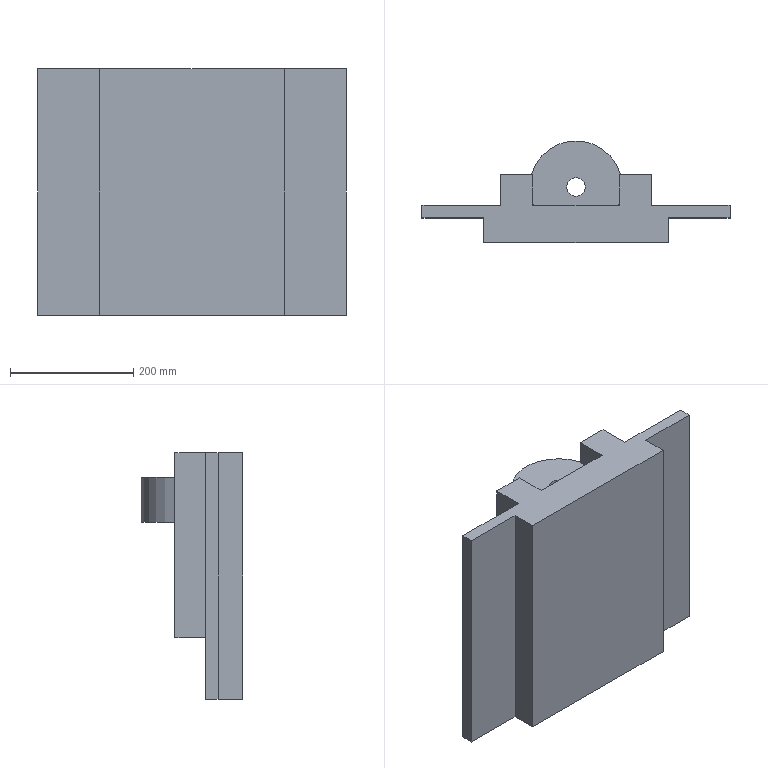Part | SolidWorks | features ICE 4, Extrusion 1 | 1 solid | 25 faces | box 500 x 165 x 400 mm | volume 11247754 mm3 | plane 20 | cylinder 5 | commonest cylinder face diameters 150 x3 30 x2
STEP:
#1=CARTESIAN_POINT('',(-15.,50.,87.));
#2=VERTEX_POINT('',#1);
#3=CARTESIAN_POINT('',(15.,50.,87.));
#4=VERTEX_POINT('',#3);
#5=CARTESIAN_POINT('',(0.,50.,87.));
#6=DIRECTION('',(0.,0.,1.));
#7=DIRECTION('',(1.,0.,0.));
#8=AXIS2_PLACEMENT_3D('',#5,#6,#7);
#9=CIRCLE('',#8,15.);
#10=EDGE_CURVE('',#2,#4,#9,.T.);
#11=ORIENTED_EDGE('',*,*,#10,.F.);
#12=CARTESIAN_POINT('',(-15.,50.,160.));
#13=VERTEX_POINT('',#12);
#14=CARTESIAN_POINT('',(-15.,50.,-200.));
#15=DIRECTION('',(0.,0.,1.));
#16=VECTOR('',#15,1000.);
#17=LINE('',#14,#16);
#18=EDGE_CURVE('',#2,#13,#17,.T.);
#19=ORIENTED_EDGE('',*,*,#18,.T.);
#20=CARTESIAN_POINT('',(15.,50.,160.));
#21=VERTEX_POINT('',#20);
#22=CARTESIAN_POINT('',(0.,50.,160.));
#23=DIRECTION('',(0.,0.,1.));
#24=DIRECTION('',(1.,0.,0.));
#25=AXIS2_PLACEMENT_3D('',#22,#23,#24);
#26=CIRCLE('',#25,15.);
#27=EDGE_CURVE('',#13,#21,#26,.T.);
#28=ORIENTED_EDGE('',*,*,#27,.T.);
#29=CARTESIAN_POINT('',(15.,50.,-200.));
#30=DIRECTION('',(0.,0.,1.));
#31=VECTOR('',#30,1000.);
#32=LINE('',#29,#31);
#33=EDGE_CURVE('',#4,#21,#32,.T.);
#34=ORIENTED_EDGE('',*,*,#33,.F.);
#35=EDGE_LOOP('',(#11,#19,#28,#34));
#36=FACE_OUTER_BOUND('',#35,.T.);
#37=CARTESIAN_POINT('',(0.,50.,-200.));
#38=DIRECTION('',(0.,0.,1.));
#39=DIRECTION('',(1.,0.,0.));
#40=AXIS2_PLACEMENT_3D('',#37,#38,#39);
#41=CYLINDRICAL_SURFACE('',#40,15.);
#42=ADVANCED_FACE('',(#36),#41,.F.);
#43=CARTESIAN_POINT('',(-250.,20.,200.));
#44=VERTEX_POINT('',#43);
#45=CARTESIAN_POINT('',(-122.,20.,200.));
#46=VERTEX_POINT('',#45);
#47=CARTESIAN_POINT('',(-250.,20.,200.));
#48=DIRECTION('',(1.,0.,0.));
#49=VECTOR('',#48,1000.);
#50=LINE('',#47,#49);
#51=EDGE_CURVE('',#44,#46,#50,.T.);
#52=ORIENTED_EDGE('',*,*,#51,.T.);
#53=CARTESIAN_POINT('',(-122.,20.,-100.));
#54=VERTEX_POINT('',#53);
#55=CARTESIAN_POINT('',(-122.,20.,-100.));
#56=DIRECTION('',(0.,0.,1.));
#57=VECTOR('',#56,1000.);
#58=LINE('',#55,#57);
#59=EDGE_CURVE('',#54,#46,#58,.T.);
#60=ORIENTED_EDGE('',*,*,#59,.F.);
#61=CARTESIAN_POINT('',(-70.,20.,-100.));
#62=VERTEX_POINT('',#61);
#63=CARTESIAN_POINT('',(-122.,20.,-100.));
#64=DIRECTION('',(-1.,0.,0.));
#65=VECTOR('',#64,1000.);
#66=LINE('',#63,#65);
#67=EDGE_CURVE('',#62,#54,#66,.T.);
#68=ORIENTED_EDGE('',*,*,#67,.F.);
#69=CARTESIAN_POINT('',(-70.,20.,200.));
#70=VERTEX_POINT('',#69);
#71=CARTESIAN_POINT('',(-70.,20.,-100.));
#72=DIRECTION('',(0.,0.,-1.));
#73=VECTOR('',#72,1000.);
#74=LINE('',#71,#73);
#75=EDGE_CURVE('',#70,#62,#74,.T.);
#76=ORIENTED_EDGE('',*,*,#75,.F.);
#77=CARTESIAN_POINT('',(70.,20.,200.));
#78=VERTEX_POINT('',#77);
#79=CARTESIAN_POINT('',(-250.,20.,200.));
#80=DIRECTION('',(1.,0.,0.));
#81=VECTOR('',#80,1000.);
#82=LINE('',#79,#81);
#83=EDGE_CURVE('',#70,#78,#82,.T.);
#84=ORIENTED_EDGE('',*,*,#83,.T.);
#85=CARTESIAN_POINT('',(70.,20.,-100.));
#86=VERTEX_POINT('',#85);
#87=CARTESIAN_POINT('',(70.,20.,-100.));
#88=DIRECTION('',(0.,0.,1.));
#89=VECTOR('',#88,1000.);
#90=LINE('',#87,#89);
#91=EDGE_CURVE('',#86,#78,#90,.T.);
#92=ORIENTED_EDGE('',*,*,#91,.F.);
#93=CARTESIAN_POINT('',(122.,20.,-100.));
#94=VERTEX_POINT('',#93);
#95=CARTESIAN_POINT('',(122.,20.,-100.));
#96=DIRECTION('',(-1.,0.,0.));
#97=VECTOR('',#96,1000.);
#98=LINE('',#95,#97);
#99=EDGE_CURVE('',#94,#86,#98,.T.);
#100=ORIENTED_EDGE('',*,*,#99,.F.);
#101=CARTESIAN_POINT('',(122.,20.,200.));
#102=VERTEX_POINT('',#101);
#103=CARTESIAN_POINT('',(122.,20.,-100.));
#104=DIRECTION('',(0.,0.,-1.));
#105=VECTOR('',#104,1000.);
#106=LINE('',#103,#105);
#107=EDGE_CURVE('',#102,#94,#106,.T.);
#108=ORIENTED_EDGE('',*,*,#107,.F.);
#109=CARTESIAN_POINT('',(250.,20.,200.));
#110=VERTEX_POINT('',#109);
#111=CARTESIAN_POINT('',(-250.,20.,200.));
#112=DIRECTION('',(1.,0.,0.));
#113=VECTOR('',#112,1000.);
#114=LINE('',#111,#113);
#115=EDGE_CURVE('',#102,#110,#114,.T.);
#116=ORIENTED_EDGE('',*,*,#115,.T.);
#117=CARTESIAN_POINT('',(250.,20.,-200.));
#118=VERTEX_POINT('',#117);
#119=CARTESIAN_POINT('',(250.,20.,-200.));
#120=DIRECTION('',(0.,0.,-1.));
#121=VECTOR('',#120,1000.);
#122=LINE('',#119,#121);
#123=EDGE_CURVE('',#110,#118,#122,.T.);
#124=ORIENTED_EDGE('',*,*,#123,.T.);
#125=CARTESIAN_POINT('',(-250.,20.,-200.));
#126=VERTEX_POINT('',#125);
#127=CARTESIAN_POINT('',(-250.,20.,-200.));
#128=DIRECTION('',(-1.,0.,0.));
#129=VECTOR('',#128,1000.);
#130=LINE('',#127,#129);
#131=EDGE_CURVE('',#118,#126,#130,.T.);
#132=ORIENTED_EDGE('',*,*,#131,.T.);
#133=CARTESIAN_POINT('',(-250.,20.,-200.));
#134=DIRECTION('',(0.,0.,1.));
#135=VECTOR('',#134,1000.);
#136=LINE('',#133,#135);
#137=EDGE_CURVE('',#126,#44,#136,.T.);
#138=ORIENTED_EDGE('',*,*,#137,.T.);
#139=EDGE_LOOP('',(#52,#60,#68,#76,#84,#92,#100,#108,#116,#124,#132,#138));
#140=FACE_OUTER_BOUND('',#139,.T.);
#141=CARTESIAN_POINT('',(-68.739,20.,87.));
#142=VERTEX_POINT('',#141);
#143=CARTESIAN_POINT('',(-68.739,20.,160.));
#144=VERTEX_POINT('',#143);
#145=CARTESIAN_POINT('',(-68.739,20.,87.));
#146=DIRECTION('',(0.,0.,1.));
#147=VECTOR('',#146,1000.);
#148=LINE('',#145,#147);
#149=EDGE_CURVE('',#142,#144,#148,.T.);
#150=ORIENTED_EDGE('',*,*,#149,.F.);
#151=CARTESIAN_POINT('',(68.739,20.,87.));
#152=VERTEX_POINT('',#151);
#153=CARTESIAN_POINT('',(0.,20.,87.));
#154=DIRECTION('',(1.,0.,0.));
#155=VECTOR('',#154,1000.);
#156=LINE('',#153,#155);
#157=EDGE_CURVE('',#142,#152,#156,.T.);
#158=ORIENTED_EDGE('',*,*,#157,.T.);
#159=CARTESIAN_POINT('',(68.739,20.,160.));
#160=VERTEX_POINT('',#159);
#161=CARTESIAN_POINT('',(68.739,20.,87.));
#162=DIRECTION('',(0.,0.,-1.));
#163=VECTOR('',#162,1000.);
#164=LINE('',#161,#163);
#165=EDGE_CURVE('',#160,#152,#164,.T.);
#166=ORIENTED_EDGE('',*,*,#165,.F.);
#167=CARTESIAN_POINT('',(0.,20.,160.));
#168=DIRECTION('',(1.,0.,0.));
#169=VECTOR('',#168,1000.);
#170=LINE('',#167,#169);
#171=EDGE_CURVE('',#144,#160,#170,.T.);
#172=ORIENTED_EDGE('',*,*,#171,.F.);
#173=EDGE_LOOP('',(#150,#158,#166,#172));
#174=FACE_BOUND('',#173,.T.);
#175=CARTESIAN_POINT('',(0.,20.,0.));
#176=DIRECTION('',(0.,1.,0.));
#177=DIRECTION('',(0.,0.,1.));
#178=AXIS2_PLACEMENT_3D('',#175,#176,#177);
#179=PLANE('',#178);
#180=ADVANCED_FACE('',(#140,#174),#179,.T.);
#181=CARTESIAN_POINT('',(70.,70.,87.));
#182=VERTEX_POINT('',#181);
#183=CARTESIAN_POINT('',(70.,23.074,87.));
#184=VERTEX_POINT('',#183);
#185=CARTESIAN_POINT('',(70.,70.,87.));
#186=DIRECTION('',(0.,-1.,0.));
#187=VECTOR('',#186,1000.);
#188=LINE('',#185,#187);
#189=EDGE_CURVE('',#182,#184,#188,.T.);
#190=ORIENTED_EDGE('',*,*,#189,.F.);
#191=CARTESIAN_POINT('',(70.,70.,-100.));
#192=VERTEX_POINT('',#191);
#193=CARTESIAN_POINT('',(70.,70.,-100.));
#194=DIRECTION('',(0.,0.,1.));
#195=VECTOR('',#194,1000.);
#196=LINE('',#193,#195);
#197=EDGE_CURVE('',#192,#182,#196,.T.);
#198=ORIENTED_EDGE('',*,*,#197,.F.);
#199=CARTESIAN_POINT('',(70.,70.,-100.));
#200=DIRECTION('',(0.,-1.,0.));
#201=VECTOR('',#200,1000.);
#202=LINE('',#199,#201);
#203=EDGE_CURVE('',#192,#86,#202,.T.);
#204=ORIENTED_EDGE('',*,*,#203,.T.);
#205=ORIENTED_EDGE('',*,*,#91,.T.);
#206=CARTESIAN_POINT('',(70.,70.,200.));
#207=VERTEX_POINT('',#206);
#208=CARTESIAN_POINT('',(70.,70.,200.));
#209=DIRECTION('',(0.,-1.,0.));
#210=VECTOR('',#209,1000.);
#211=LINE('',#208,#210);
#212=EDGE_CURVE('',#207,#78,#211,.T.);
#213=ORIENTED_EDGE('',*,*,#212,.F.);
#214=CARTESIAN_POINT('',(70.,70.,160.));
#215=VERTEX_POINT('',#214);
#216=CARTESIAN_POINT('',(70.,70.,-100.));
#217=DIRECTION('',(0.,0.,1.));
#218=VECTOR('',#217,1000.);
#219=LINE('',#216,#218);
#220=EDGE_CURVE('',#215,#207,#219,.T.);
#221=ORIENTED_EDGE('',*,*,#220,.F.);
#222=CARTESIAN_POINT('',(70.,23.074,160.));
#223=VERTEX_POINT('',#222);
#224=CARTESIAN_POINT('',(70.,70.,160.));
#225=DIRECTION('',(0.,-1.,0.));
#226=VECTOR('',#225,1000.);
#227=LINE('',#224,#226);
#228=EDGE_CURVE('',#215,#223,#227,.T.);
#229=ORIENTED_EDGE('',*,*,#228,.T.);
#230=CARTESIAN_POINT('',(70.,23.074,87.));
#231=DIRECTION('',(0.,0.,-1.));
#232=VECTOR('',#231,1000.);
#233=LINE('',#230,#232);
#234=EDGE_CURVE('',#223,#184,#233,.T.);
#235=ORIENTED_EDGE('',*,*,#234,.T.);
#236=EDGE_LOOP('',(#190,#198,#204,#205,#213,#221,#229,#235));
#237=FACE_OUTER_BOUND('',#236,.T.);
#238=CARTESIAN_POINT('',(70.,70.,-100.));
#239=DIRECTION('',(1.,0.,0.));
#240=DIRECTION('',(0.,0.,-1.));
#241=AXIS2_PLACEMENT_3D('',#238,#239,#240);
#242=PLANE('',#241);
#243=ADVANCED_FACE('',(#237),#242,.F.);
#244=CARTESIAN_POINT('',(72.284,70.,87.));
#245=VERTEX_POINT('',#244);
#246=CARTESIAN_POINT('',(0.,70.,87.));
#247=DIRECTION('',(-1.,0.,0.));
#248=VECTOR('',#247,1000.);
#249=LINE('',#246,#248);
#250=EDGE_CURVE('',#245,#182,#249,.T.);
#251=ORIENTED_EDGE('',*,*,#250,.F.);
#252=CARTESIAN_POINT('',(72.284,70.,160.));
#253=VERTEX_POINT('',#252);
#254=CARTESIAN_POINT('',(72.284,70.,87.));
#255=DIRECTION('',(0.,0.,1.));
#256=VECTOR('',#255,1000.);
#257=LINE('',#254,#256);
#258=EDGE_CURVE('',#245,#253,#257,.T.);
#259=ORIENTED_EDGE('',*,*,#258,.T.);
#260=CARTESIAN_POINT('',(0.,70.,160.));
#261=DIRECTION('',(-1.,0.,0.));
#262=VECTOR('',#261,1000.);
#263=LINE('',#260,#262);
#264=EDGE_CURVE('',#253,#215,#263,.T.);
#265=ORIENTED_EDGE('',*,*,#264,.T.);
#266=ORIENTED_EDGE('',*,*,#220,.T.);
#267=CARTESIAN_POINT('',(122.,70.,200.));
#268=VERTEX_POINT('',#267);
#269=CARTESIAN_POINT('',(122.,70.,200.));
#270=DIRECTION('',(1.,0.,0.));
#271=VECTOR('',#270,1000.);
#272=LINE('',#269,#271);
#273=EDGE_CURVE('',#207,#268,#272,.T.);
#274=ORIENTED_EDGE('',*,*,#273,.T.);
#275=CARTESIAN_POINT('',(122.,70.,-100.));
#276=VERTEX_POINT('',#275);
#277=CARTESIAN_POINT('',(122.,70.,-100.));
#278=DIRECTION('',(0.,0.,-1.));
#279=VECTOR('',#278,1000.);
#280=LINE('',#277,#279);
#281=EDGE_CURVE('',#268,#276,#280,.T.);
#282=ORIENTED_EDGE('',*,*,#281,.T.);
#283=CARTESIAN_POINT('',(122.,70.,-100.));
#284=DIRECTION('',(-1.,0.,0.));
#285=VECTOR('',#284,1000.);
#286=LINE('',#283,#285);
#287=EDGE_CURVE('',#276,#192,#286,.T.);
#288=ORIENTED_EDGE('',*,*,#287,.T.);
#289=ORIENTED_EDGE('',*,*,#197,.T.);
#290=EDGE_LOOP('',(#251,#259,#265,#266,#274,#282,#288,#289));
#291=FACE_OUTER_BOUND('',#290,.T.);
#292=CARTESIAN_POINT('',(0.,70.,0.));
#293=DIRECTION('',(0.,-1.,0.));
#294=DIRECTION('',(0.,0.,-1.));
#295=AXIS2_PLACEMENT_3D('',#292,#293,#294);
#296=PLANE('',#295);
#297=ADVANCED_FACE('',(#291),#296,.F.);
#298=CARTESIAN_POINT('',(-70.,23.074,87.));
#299=VERTEX_POINT('',#298);
#300=CARTESIAN_POINT('',(-70.,70.,87.));
#301=VERTEX_POINT('',#300);
#302=CARTESIAN_POINT('',(-70.,70.,87.));
#303=DIRECTION('',(0.,1.,0.));
#304=VECTOR('',#303,1000.);
#305=LINE('',#302,#304);
#306=EDGE_CURVE('',#299,#301,#305,.T.);
#307=ORIENTED_EDGE('',*,*,#306,.F.);
#308=CARTESIAN_POINT('',(-70.,23.074,160.));
#309=VERTEX_POINT('',#308);
#310=CARTESIAN_POINT('',(-70.,23.074,87.));
#311=DIRECTION('',(0.,0.,1.));
#312=VECTOR('',#311,1000.);
#313=LINE('',#310,#312);
#314=EDGE_CURVE('',#299,#309,#313,.T.);
#315=ORIENTED_EDGE('',*,*,#314,.T.);
#316=CARTESIAN_POINT('',(-70.,70.,160.));
#317=VERTEX_POINT('',#316);
#318=CARTESIAN_POINT('',(-70.,70.,160.));
#319=DIRECTION('',(0.,1.,0.));
#320=VECTOR('',#319,1000.);
#321=LINE('',#318,#320);
#322=EDGE_CURVE('',#309,#317,#321,.T.);
#323=ORIENTED_EDGE('',*,*,#322,.T.);
#324=CARTESIAN_POINT('',(-70.,70.,200.));
#325=VERTEX_POINT('',#324);
#326=CARTESIAN_POINT('',(-70.,70.,-100.));
#327=DIRECTION('',(0.,0.,-1.));
#328=VECTOR('',#327,1000.);
#329=LINE('',#326,#328);
#330=EDGE_CURVE('',#325,#317,#329,.T.);
#331=ORIENTED_EDGE('',*,*,#330,.F.);
#332=CARTESIAN_POINT('',(-70.,70.,200.));
#333=DIRECTION('',(0.,-1.,0.));
#334=VECTOR('',#333,1000.);
#335=LINE('',#332,#334);
#336=EDGE_CURVE('',#325,#70,#335,.T.);
#337=ORIENTED_EDGE('',*,*,#336,.T.);
#338=ORIENTED_EDGE('',*,*,#75,.T.);
#339=CARTESIAN_POINT('',(-70.,70.,-100.));
#340=VERTEX_POINT('',#339);
#341=CARTESIAN_POINT('',(-70.,70.,-100.));
#342=DIRECTION('',(0.,-1.,0.));
#343=VECTOR('',#342,1000.);
#344=LINE('',#341,#343);
#345=EDGE_CURVE('',#340,#62,#344,.T.);
#346=ORIENTED_EDGE('',*,*,#345,.F.);
#347=CARTESIAN_POINT('',(-70.,70.,-100.));
#348=DIRECTION('',(0.,0.,-1.));
#349=VECTOR('',#348,1000.);
#350=LINE('',#347,#349);
#351=EDGE_CURVE('',#301,#340,#350,.T.);
#352=ORIENTED_EDGE('',*,*,#351,.F.);
#353=EDGE_LOOP('',(#307,#315,#323,#331,#337,#338,#346,#352));
#354=FACE_OUTER_BOUND('',#353,.T.);
#355=CARTESIAN_POINT('',(-70.,70.,-100.));
#356=DIRECTION('',(-1.,0.,0.));
#357=DIRECTION('',(0.,0.,1.));
#358=AXIS2_PLACEMENT_3D('',#355,#356,#357);
#359=PLANE('',#358);
#360=ADVANCED_FACE('',(#354),#359,.F.);
#361=CARTESIAN_POINT('',(-72.284,70.,87.));
#362=VERTEX_POINT('',#361);
#363=CARTESIAN_POINT('',(0.,70.,87.));
#364=DIRECTION('',(-1.,0.,0.));
#365=VECTOR('',#364,1000.);
#366=LINE('',#363,#365);
#367=EDGE_CURVE('',#301,#362,#366,.T.);
#368=ORIENTED_EDGE('',*,*,#367,.F.);
#369=ORIENTED_EDGE('',*,*,#351,.T.);
#370=CARTESIAN_POINT('',(-122.,70.,-100.));
#371=VERTEX_POINT('',#370);
#372=CARTESIAN_POINT('',(-122.,70.,-100.));
#373=DIRECTION('',(-1.,0.,0.));
#374=VECTOR('',#373,1000.);
#375=LINE('',#372,#374);
#376=EDGE_CURVE('',#340,#371,#375,.T.);
#377=ORIENTED_EDGE('',*,*,#376,.T.);
#378=CARTESIAN_POINT('',(-122.,70.,200.));
#379=VERTEX_POINT('',#378);
#380=CARTESIAN_POINT('',(-122.,70.,-100.));
#381=DIRECTION('',(0.,0.,1.));
#382=VECTOR('',#381,1000.);
#383=LINE('',#380,#382);
#384=EDGE_CURVE('',#371,#379,#383,.T.);
#385=ORIENTED_EDGE('',*,*,#384,.T.);
#386=CARTESIAN_POINT('',(-122.,70.,200.));
#387=DIRECTION('',(1.,0.,0.));
#388=VECTOR('',#387,1000.);
#389=LINE('',#386,#388);
#390=EDGE_CURVE('',#379,#325,#389,.T.);
#391=ORIENTED_EDGE('',*,*,#390,.T.);
#392=ORIENTED_EDGE('',*,*,#330,.T.);
#393=CARTESIAN_POINT('',(-72.284,70.,160.));
#394=VERTEX_POINT('',#393);
#395=CARTESIAN_POINT('',(0.,70.,160.));
#396=DIRECTION('',(-1.,0.,0.));
#397=VECTOR('',#396,1000.);
#398=LINE('',#395,#397);
#399=EDGE_CURVE('',#317,#394,#398,.T.);
#400=ORIENTED_EDGE('',*,*,#399,.T.);
#401=CARTESIAN_POINT('',(-72.284,70.,87.));
#402=DIRECTION('',(0.,0.,-1.));
#403=VECTOR('',#402,1000.);
#404=LINE('',#401,#403);
#405=EDGE_CURVE('',#394,#362,#404,.T.);
#406=ORIENTED_EDGE('',*,*,#405,.T.);
#407=EDGE_LOOP('',(#368,#369,#377,#385,#391,#392,#400,#406));
#408=FACE_OUTER_BOUND('',#407,.T.);
#409=CARTESIAN_POINT('',(0.,70.,0.));
#410=DIRECTION('',(0.,-1.,0.));
#411=DIRECTION('',(0.,0.,-1.));
#412=AXIS2_PLACEMENT_3D('',#409,#410,#411);
#413=PLANE('',#412);
#414=ADVANCED_FACE('',(#408),#413,.F.);
#415=CARTESIAN_POINT('',(150.,0.,-200.));
#416=VERTEX_POINT('',#415);
#417=CARTESIAN_POINT('',(150.,0.,200.));
#418=VERTEX_POINT('',#417);
#419=CARTESIAN_POINT('',(150.,0.,-200.));
#420=DIRECTION('',(0.,0.,1.));
#421=VECTOR('',#420,1000.);
#422=LINE('',#419,#421);
#423=EDGE_CURVE('',#416,#418,#422,.T.);
#424=ORIENTED_EDGE('',*,*,#423,.F.);
#425=CARTESIAN_POINT('',(250.,0.,-200.));
#426=VERTEX_POINT('',#425);
#427=CARTESIAN_POINT('',(-250.,0.,-200.));
#428=DIRECTION('',(-1.,0.,0.));
#429=VECTOR('',#428,1000.);
#430=LINE('',#427,#429);
#431=EDGE_CURVE('',#426,#416,#430,.T.);
#432=ORIENTED_EDGE('',*,*,#431,.F.);
#433=CARTESIAN_POINT('',(250.,0.,200.));
#434=VERTEX_POINT('',#433);
#435=CARTESIAN_POINT('',(250.,0.,-200.));
#436=DIRECTION('',(0.,0.,-1.));
#437=VECTOR('',#436,1000.);
#438=LINE('',#435,#437);
#439=EDGE_CURVE('',#434,#426,#438,.T.);
#440=ORIENTED_EDGE('',*,*,#439,.F.);
#441=CARTESIAN_POINT('',(-250.,0.,200.));
#442=DIRECTION('',(1.,0.,0.));
#443=VECTOR('',#442,1000.);
#444=LINE('',#441,#443);
#445=EDGE_CURVE('',#418,#434,#444,.T.);
#446=ORIENTED_EDGE('',*,*,#445,.F.);
#447=EDGE_LOOP('',(#424,#432,#440,#446));
#448=FACE_OUTER_BOUND('',#447,.T.);
#449=CARTESIAN_POINT('',(0.,0.,0.));
#450=DIRECTION('',(0.,1.,0.));
#451=DIRECTION('',(0.,0.,1.));
#452=AXIS2_PLACEMENT_3D('',#449,#450,#451);
#453=PLANE('',#452);
#454=ADVANCED_FACE('',(#448),#453,.F.);
#455=CARTESIAN_POINT('',(-150.,0.,200.));
#456=VERTEX_POINT('',#455);
#457=CARTESIAN_POINT('',(-150.,0.,-200.));
#458=VERTEX_POINT('',#457);
#459=CARTESIAN_POINT('',(-150.,0.,-200.));
#460=DIRECTION('',(0.,0.,-1.));
#461=VECTOR('',#460,1000.);
#462=LINE('',#459,#461);
#463=EDGE_CURVE('',#456,#458,#462,.T.);
#464=ORIENTED_EDGE('',*,*,#463,.F.);
#465=CARTESIAN_POINT('',(-250.,0.,200.));
#466=VERTEX_POINT('',#465);
#467=CARTESIAN_POINT('',(-250.,0.,200.));
#468=DIRECTION('',(1.,0.,0.));
#469=VECTOR('',#468,1000.);
#470=LINE('',#467,#469);
#471=EDGE_CURVE('',#466,#456,#470,.T.);
#472=ORIENTED_EDGE('',*,*,#471,.F.);
#473=CARTESIAN_POINT('',(-250.,0.,-200.));
#474=VERTEX_POINT('',#473);
#475=CARTESIAN_POINT('',(-250.,0.,-200.));
#476=DIRECTION('',(0.,0.,1.));
#477=VECTOR('',#476,1000.);
#478=LINE('',#475,#477);
#479=EDGE_CURVE('',#474,#466,#478,.T.);
#480=ORIENTED_EDGE('',*,*,#479,.F.);
#481=CARTESIAN_POINT('',(-250.,0.,-200.));
#482=DIRECTION('',(-1.,0.,0.));
#483=VECTOR('',#482,1000.);
#484=LINE('',#481,#483);
#485=EDGE_CURVE('',#458,#474,#484,.T.);
#486=ORIENTED_EDGE('',*,*,#485,.F.);
#487=EDGE_LOOP('',(#464,#472,#480,#486));
#488=FACE_OUTER_BOUND('',#487,.T.);
#489=CARTESIAN_POINT('',(0.,0.,0.));
#490=DIRECTION('',(0.,1.,0.));
#491=DIRECTION('',(0.,0.,1.));
#492=AXIS2_PLACEMENT_3D('',#489,#490,#491);
#493=PLANE('',#492);
#494=ADVANCED_FACE('',(#488),#493,.F.);
#495=ORIENTED_EDGE('',*,*,#439,.T.);
#496=CARTESIAN_POINT('',(250.,20.,-200.));
#497=DIRECTION('',(0.,-1.,0.));
#498=VECTOR('',#497,1000.);
#499=LINE('',#496,#498);
#500=EDGE_CURVE('',#118,#426,#499,.T.);
#501=ORIENTED_EDGE('',*,*,#500,.F.);
#502=ORIENTED_EDGE('',*,*,#123,.F.);
#503=CARTESIAN_POINT('',(250.,20.,200.));
#504=DIRECTION('',(0.,-1.,0.));
#505=VECTOR('',#504,1000.);
#506=LINE('',#503,#505);
#507=EDGE_CURVE('',#110,#434,#506,.T.);
#508=ORIENTED_EDGE('',*,*,#507,.T.);
#509=EDGE_LOOP('',(#495,#501,#502,#508));
#510=FACE_OUTER_BOUND('',#509,.T.);
#511=CARTESIAN_POINT('',(250.,20.,-200.));
#512=DIRECTION('',(-1.,0.,0.));
#513=DIRECTION('',(0.,0.,1.));
#514=AXIS2_PLACEMENT_3D('',#511,#512,#513);
#515=PLANE('',#514);
#516=ADVANCED_FACE('',(#510),#515,.F.);
#517=ORIENTED_EDGE('',*,*,#431,.T.);
#518=CARTESIAN_POINT('',(150.,-40.,-200.));
#519=VERTEX_POINT('',#518);
#520=CARTESIAN_POINT('',(150.,-40.,-200.));
#521=DIRECTION('',(0.,1.,0.));
#522=VECTOR('',#521,1000.);
#523=LINE('',#520,#522);
#524=EDGE_CURVE('',#519,#416,#523,.T.);
#525=ORIENTED_EDGE('',*,*,#524,.F.);
#526=CARTESIAN_POINT('',(-150.,-40.,-200.));
#527=VERTEX_POINT('',#526);
#528=CARTESIAN_POINT('',(-150.,-40.,-200.));
#529=DIRECTION('',(1.,0.,0.));
#530=VECTOR('',#529,1000.);
#531=LINE('',#528,#530);
#532=EDGE_CURVE('',#527,#519,#531,.T.);
#533=ORIENTED_EDGE('',*,*,#532,.F.);
#534=CARTESIAN_POINT('',(-150.,-40.,-200.));
#535=DIRECTION('',(0.,1.,0.));
#536=VECTOR('',#535,1000.);
#537=LINE('',#534,#536);
#538=EDGE_CURVE('',#527,#458,#537,.T.);
#539=ORIENTED_EDGE('',*,*,#538,.T.);
#540=ORIENTED_EDGE('',*,*,#485,.T.);
#541=CARTESIAN_POINT('',(-250.,20.,-200.));
#542=DIRECTION('',(0.,-1.,0.));
#543=VECTOR('',#542,1000.);
#544=LINE('',#541,#543);
#545=EDGE_CURVE('',#126,#474,#544,.T.);
#546=ORIENTED_EDGE('',*,*,#545,.F.);
#547=ORIENTED_EDGE('',*,*,#131,.F.);
#548=ORIENTED_EDGE('',*,*,#500,.T.);
#549=EDGE_LOOP('',(#517,#525,#533,#539,#540,#546,#547,#548));
#550=FACE_OUTER_BOUND('',#549,.T.);
#551=CARTESIAN_POINT('',(-250.,20.,-200.));
#552=DIRECTION('',(0.,0.,1.));
#553=DIRECTION('',(1.,0.,0.));
#554=AXIS2_PLACEMENT_3D('',#551,#552,#553);
#555=PLANE('',#554);
#556=ADVANCED_FACE('',(#550),#555,.F.);
#557=ORIENTED_EDGE('',*,*,#479,.T.);
#558=CARTESIAN_POINT('',(-250.,20.,200.));
#559=DIRECTION('',(0.,-1.,0.));
#560=VECTOR('',#559,1000.);
#561=LINE('',#558,#560);
#562=EDGE_CURVE('',#44,#466,#561,.T.);
#563=ORIENTED_EDGE('',*,*,#562,.F.);
#564=ORIENTED_EDGE('',*,*,#137,.F.);
#565=ORIENTED_EDGE('',*,*,#545,.T.);
#566=EDGE_LOOP('',(#557,#563,#564,#565));
#567=FACE_OUTER_BOUND('',#566,.T.);
#568=CARTESIAN_POINT('',(-250.,20.,-200.));
#569=DIRECTION('',(1.,0.,0.));
#570=DIRECTION('',(0.,0.,-1.));
#571=AXIS2_PLACEMENT_3D('',#568,#569,#570);
#572=PLANE('',#571);
#573=ADVANCED_FACE('',(#567),#572,.F.);
#574=ORIENTED_EDGE('',*,*,#471,.T.);
#575=CARTESIAN_POINT('',(-150.,-40.,200.));
#576=VERTEX_POINT('',#575);
#577=CARTESIAN_POINT('',(-150.,-40.,200.));
#578=DIRECTION('',(0.,1.,0.));
#579=VECTOR('',#578,1000.);
#580=LINE('',#577,#579);
#581=EDGE_CURVE('',#576,#456,#580,.T.);
#582=ORIENTED_EDGE('',*,*,#581,.F.);
#583=CARTESIAN_POINT('',(150.,-40.,200.));
#584=VERTEX_POINT('',#583);
#585=CARTESIAN_POINT('',(-150.,-40.,200.));
#586=DIRECTION('',(-1.,0.,0.));
#587=VECTOR('',#586,1000.);
#588=LINE('',#585,#587);
#589=EDGE_CURVE('',#584,#576,#588,.T.);
#590=ORIENTED_EDGE('',*,*,#589,.F.);
#591=CARTESIAN_POINT('',(150.,-40.,200.));
#592=DIRECTION('',(0.,1.,0.));
#593=VECTOR('',#592,1000.);
#594=LINE('',#591,#593);
#595=EDGE_CURVE('',#584,#418,#594,.T.);
#596=ORIENTED_EDGE('',*,*,#595,.T.);
#597=ORIENTED_EDGE('',*,*,#445,.T.);
#598=ORIENTED_EDGE('',*,*,#507,.F.);
#599=ORIENTED_EDGE('',*,*,#115,.F.);
#600=CARTESIAN_POINT('',(122.,70.,200.));
#601=DIRECTION('',(0.,-1.,0.));
#602=VECTOR('',#601,1000.);
#603=LINE('',#600,#602);
#604=EDGE_CURVE('',#268,#102,#603,.T.);
#605=ORIENTED_EDGE('',*,*,#604,.F.);
#606=ORIENTED_EDGE('',*,*,#273,.F.);
#607=ORIENTED_EDGE('',*,*,#212,.T.);
#608=ORIENTED_EDGE('',*,*,#83,.F.);
#609=ORIENTED_EDGE('',*,*,#336,.F.);
#610=ORIENTED_EDGE('',*,*,#390,.F.);
#611=CARTESIAN_POINT('',(-122.,70.,200.));
#612=DIRECTION('',(0.,-1.,0.));
#613=VECTOR('',#612,1000.);
#614=LINE('',#611,#613);
#615=EDGE_CURVE('',#379,#46,#614,.T.);
#616=ORIENTED_EDGE('',*,*,#615,.T.);
#617=ORIENTED_EDGE('',*,*,#51,.F.);
#618=ORIENTED_EDGE('',*,*,#562,.T.);
#619=EDGE_LOOP('',(#574,#582,#590,#596,#597,#598,#599,#605,#606,#607,#608,#609,#610,#616,#617,#618));
#620=FACE_OUTER_BOUND('',#619,.T.);
#621=CARTESIAN_POINT('',(-250.,20.,200.));
#622=DIRECTION('',(0.,0.,-1.));
#623=DIRECTION('',(-1.,0.,0.));
#624=AXIS2_PLACEMENT_3D('',#621,#622,#623);
#625=PLANE('',#624);
#626=ADVANCED_FACE('',(#620),#625,.F.);
#627=ORIENTED_EDGE('',*,*,#107,.T.);
#628=CARTESIAN_POINT('',(122.,70.,-100.));
#629=DIRECTION('',(0.,-1.,0.));
#630=VECTOR('',#629,1000.);
#631=LINE('',#628,#630);
#632=EDGE_CURVE('',#276,#94,#631,.T.);
#633=ORIENTED_EDGE('',*,*,#632,.F.);
#634=ORIENTED_EDGE('',*,*,#281,.F.);
#635=ORIENTED_EDGE('',*,*,#604,.T.);
#636=EDGE_LOOP('',(#627,#633,#634,#635));
#637=FACE_OUTER_BOUND('',#636,.T.);
#638=CARTESIAN_POINT('',(122.,70.,-100.));
#639=DIRECTION('',(-1.,0.,0.));
#640=DIRECTION('',(0.,0.,1.));
#641=AXIS2_PLACEMENT_3D('',#638,#639,#640);
#642=PLANE('',#641);
#643=ADVANCED_FACE('',(#637),#642,.F.);
#644=ORIENTED_EDGE('',*,*,#99,.T.);
#645=ORIENTED_EDGE('',*,*,#203,.F.);
#646=ORIENTED_EDGE('',*,*,#287,.F.);
#647=ORIENTED_EDGE('',*,*,#632,.T.);
#648=EDGE_LOOP('',(#644,#645,#646,#647));
#649=FACE_OUTER_BOUND('',#648,.T.);
#650=CARTESIAN_POINT('',(122.,70.,-100.));
#651=DIRECTION('',(0.,0.,1.));
#652=DIRECTION('',(1.,0.,0.));
#653=AXIS2_PLACEMENT_3D('',#650,#651,#652);
#654=PLANE('',#653);
#655=ADVANCED_FACE('',(#649),#654,.F.);
#656=ORIENTED_EDGE('',*,*,#67,.T.);
#657=CARTESIAN_POINT('',(-122.,70.,-100.));
#658=DIRECTION('',(0.,-1.,0.));
#659=VECTOR('',#658,1000.);
#660=LINE('',#657,#659);
#661=EDGE_CURVE('',#371,#54,#660,.T.);
#662=ORIENTED_EDGE('',*,*,#661,.F.);
#663=ORIENTED_EDGE('',*,*,#376,.F.);
#664=ORIENTED_EDGE('',*,*,#345,.T.);
#665=EDGE_LOOP('',(#656,#662,#663,#664));
#666=FACE_OUTER_BOUND('',#665,.T.);
#667=CARTESIAN_POINT('',(-122.,70.,-100.));
#668=DIRECTION('',(0.,0.,1.));
#669=DIRECTION('',(1.,0.,0.));
#670=AXIS2_PLACEMENT_3D('',#667,#668,#669);
#671=PLANE('',#670);
#672=ADVANCED_FACE('',(#666),#671,.F.);
#673=ORIENTED_EDGE('',*,*,#59,.T.);
#674=ORIENTED_EDGE('',*,*,#615,.F.);
#675=ORIENTED_EDGE('',*,*,#384,.F.);
#676=ORIENTED_EDGE('',*,*,#661,.T.);
#677=EDGE_LOOP('',(#673,#674,#675,#676));
#678=FACE_OUTER_BOUND('',#677,.T.);
#679=CARTESIAN_POINT('',(-122.,70.,-100.));
#680=DIRECTION('',(1.,0.,0.));
#681=DIRECTION('',(0.,0.,-1.));
#682=AXIS2_PLACEMENT_3D('',#679,#680,#681);
#683=PLANE('',#682);
#684=ADVANCED_FACE('',(#678),#683,.F.);
#685=ORIENTED_EDGE('',*,*,#423,.T.);
#686=ORIENTED_EDGE('',*,*,#595,.F.);
#687=CARTESIAN_POINT('',(150.,-40.,-200.));
#688=DIRECTION('',(0.,0.,1.));
#689=VECTOR('',#688,1000.);
#690=LINE('',#687,#689);
#691=EDGE_CURVE('',#519,#584,#690,.T.);
#692=ORIENTED_EDGE('',*,*,#691,.F.);
#693=ORIENTED_EDGE('',*,*,#524,.T.);
#694=EDGE_LOOP('',(#685,#686,#692,#693));
#695=FACE_OUTER_BOUND('',#694,.T.);
#696=CARTESIAN_POINT('',(150.,-40.,-200.));
#697=DIRECTION('',(-1.,0.,0.));
#698=DIRECTION('',(0.,0.,1.));
#699=AXIS2_PLACEMENT_3D('',#696,#697,#698);
#700=PLANE('',#699);
#701=ADVANCED_FACE('',(#695),#700,.F.);
#702=ORIENTED_EDGE('',*,*,#463,.T.);
#703=ORIENTED_EDGE('',*,*,#538,.F.);
#704=CARTESIAN_POINT('',(-150.,-40.,-200.));
#705=DIRECTION('',(0.,0.,-1.));
#706=VECTOR('',#705,1000.);
#707=LINE('',#704,#706);
#708=EDGE_CURVE('',#576,#527,#707,.T.);
#709=ORIENTED_EDGE('',*,*,#708,.F.);
#710=ORIENTED_EDGE('',*,*,#581,.T.);
#711=EDGE_LOOP('',(#702,#703,#709,#710));
#712=FACE_OUTER_BOUND('',#711,.T.);
#713=CARTESIAN_POINT('',(-150.,-40.,-200.));
#714=DIRECTION('',(1.,0.,0.));
#715=DIRECTION('',(0.,0.,-1.));
#716=AXIS2_PLACEMENT_3D('',#713,#714,#715);
#717=PLANE('',#716);
#718=ADVANCED_FACE('',(#712),#717,.F.);
#719=ORIENTED_EDGE('',*,*,#691,.T.);
#720=ORIENTED_EDGE('',*,*,#589,.T.);
#721=ORIENTED_EDGE('',*,*,#708,.T.);
#722=ORIENTED_EDGE('',*,*,#532,.T.);
#723=EDGE_LOOP('',(#719,#720,#721,#722));
#724=FACE_OUTER_BOUND('',#723,.T.);
#725=CARTESIAN_POINT('',(0.,-40.,0.));
#726=DIRECTION('',(0.,1.,0.));
#727=DIRECTION('',(0.,0.,1.));
#728=AXIS2_PLACEMENT_3D('',#725,#726,#727);
#729=PLANE('',#728);
#730=ADVANCED_FACE('',(#724),#729,.F.);
#731=CARTESIAN_POINT('',(0.,50.,87.));
#732=DIRECTION('',(0.,0.,1.));
#733=DIRECTION('',(1.,0.,0.));
#734=AXIS2_PLACEMENT_3D('',#731,#732,#733);
#735=CIRCLE('',#734,75.);
#736=EDGE_CURVE('',#299,#142,#735,.T.);
#737=ORIENTED_EDGE('',*,*,#736,.T.);
#738=ORIENTED_EDGE('',*,*,#149,.T.);
#739=CARTESIAN_POINT('',(0.,50.,160.));
#740=DIRECTION('',(0.,0.,1.));
#741=DIRECTION('',(1.,0.,0.));
#742=AXIS2_PLACEMENT_3D('',#739,#740,#741);
#743=CIRCLE('',#742,75.);
#744=EDGE_CURVE('',#309,#144,#743,.T.);
#745=ORIENTED_EDGE('',*,*,#744,.F.);
#746=ORIENTED_EDGE('',*,*,#314,.F.);
#747=EDGE_LOOP('',(#737,#738,#745,#746));
#748=FACE_OUTER_BOUND('',#747,.T.);
#749=CARTESIAN_POINT('',(0.,50.,87.));
#750=DIRECTION('',(0.,0.,1.));
#751=DIRECTION('',(1.,0.,0.));
#752=AXIS2_PLACEMENT_3D('',#749,#750,#751);
#753=CYLINDRICAL_SURFACE('',#752,75.);
#754=ADVANCED_FACE('',(#748),#753,.T.);
#755=CARTESIAN_POINT('',(0.,50.,160.));
#756=DIRECTION('',(0.,0.,1.));
#757=DIRECTION('',(1.,0.,0.));
#758=AXIS2_PLACEMENT_3D('',#755,#756,#757);
#759=CIRCLE('',#758,75.);
#760=EDGE_CURVE('',#160,#223,#759,.T.);
#761=ORIENTED_EDGE('',*,*,#760,.F.);
#762=ORIENTED_EDGE('',*,*,#165,.T.);
#763=CARTESIAN_POINT('',(0.,50.,87.));
#764=DIRECTION('',(0.,0.,1.));
#765=DIRECTION('',(1.,0.,0.));
#766=AXIS2_PLACEMENT_3D('',#763,#764,#765);
#767=CIRCLE('',#766,75.);
#768=EDGE_CURVE('',#152,#184,#767,.T.);
#769=ORIENTED_EDGE('',*,*,#768,.T.);
#770=ORIENTED_EDGE('',*,*,#234,.F.);
#771=EDGE_LOOP('',(#761,#762,#769,#770));
#772=FACE_OUTER_BOUND('',#771,.T.);
#773=CARTESIAN_POINT('',(0.,50.,87.));
#774=DIRECTION('',(0.,0.,1.));
#775=DIRECTION('',(1.,0.,0.));
#776=AXIS2_PLACEMENT_3D('',#773,#774,#775);
#777=CYLINDRICAL_SURFACE('',#776,75.);
#778=ADVANCED_FACE('',(#772),#777,.T.);
#779=ORIENTED_EDGE('',*,*,#258,.F.);
#780=CARTESIAN_POINT('',(0.,50.,87.));
#781=DIRECTION('',(0.,0.,1.));
#782=DIRECTION('',(1.,0.,0.));
#783=AXIS2_PLACEMENT_3D('',#780,#781,#782);
#784=CIRCLE('',#783,75.);
#785=EDGE_CURVE('',#245,#362,#784,.T.);
#786=ORIENTED_EDGE('',*,*,#785,.T.);
#787=ORIENTED_EDGE('',*,*,#405,.F.);
#788=CARTESIAN_POINT('',(0.,50.,160.));
#789=DIRECTION('',(0.,0.,1.));
#790=DIRECTION('',(1.,0.,0.));
#791=AXIS2_PLACEMENT_3D('',#788,#789,#790);
#792=CIRCLE('',#791,75.);
#793=EDGE_CURVE('',#253,#394,#792,.T.);
#794=ORIENTED_EDGE('',*,*,#793,.F.);
#795=EDGE_LOOP('',(#779,#786,#787,#794));
#796=FACE_OUTER_BOUND('',#795,.T.);
#797=CARTESIAN_POINT('',(0.,50.,87.));
#798=DIRECTION('',(0.,0.,1.));
#799=DIRECTION('',(1.,0.,0.));
#800=AXIS2_PLACEMENT_3D('',#797,#798,#799);
#801=CYLINDRICAL_SURFACE('',#800,75.);
#802=ADVANCED_FACE('',(#796),#801,.T.);
#803=CARTESIAN_POINT('',(0.,50.,87.));
#804=DIRECTION('',(0.,0.,1.));
#805=DIRECTION('',(1.,0.,0.));
#806=AXIS2_PLACEMENT_3D('',#803,#804,#805);
#807=CIRCLE('',#806,15.);
#808=EDGE_CURVE('',#4,#2,#807,.T.);
#809=ORIENTED_EDGE('',*,*,#808,.T.);
#810=ORIENTED_EDGE('',*,*,#10,.T.);
#811=EDGE_LOOP('',(#809,#810));
#812=FACE_BOUND('',#811,.T.);
#813=ORIENTED_EDGE('',*,*,#157,.F.);
#814=ORIENTED_EDGE('',*,*,#736,.F.);
#815=ORIENTED_EDGE('',*,*,#306,.T.);
#816=ORIENTED_EDGE('',*,*,#367,.T.);
#817=ORIENTED_EDGE('',*,*,#785,.F.);
#818=ORIENTED_EDGE('',*,*,#250,.T.);
#819=ORIENTED_EDGE('',*,*,#189,.T.);
#820=ORIENTED_EDGE('',*,*,#768,.F.);
#821=EDGE_LOOP('',(#813,#814,#815,#816,#817,#818,#819,#820));
#822=FACE_OUTER_BOUND('',#821,.T.);
#823=CARTESIAN_POINT('',(0.,50.,87.));
#824=DIRECTION('',(0.,0.,1.));
#825=DIRECTION('',(1.,0.,0.));
#826=AXIS2_PLACEMENT_3D('',#823,#824,#825);
#827=PLANE('',#826);
#828=ADVANCED_FACE('',(#812,#822),#827,.F.);
#829=CARTESIAN_POINT('',(0.,50.,160.));
#830=DIRECTION('',(0.,0.,1.));
#831=DIRECTION('',(1.,0.,0.));
#832=AXIS2_PLACEMENT_3D('',#829,#830,#831);
#833=CIRCLE('',#832,15.);
#834=EDGE_CURVE('',#21,#13,#833,.T.);
#835=ORIENTED_EDGE('',*,*,#834,.F.);
#836=ORIENTED_EDGE('',*,*,#27,.F.);
#837=EDGE_LOOP('',(#835,#836));
#838=FACE_BOUND('',#837,.T.);
#839=ORIENTED_EDGE('',*,*,#744,.T.);
#840=ORIENTED_EDGE('',*,*,#171,.T.);
#841=ORIENTED_EDGE('',*,*,#760,.T.);
#842=ORIENTED_EDGE('',*,*,#228,.F.);
#843=ORIENTED_EDGE('',*,*,#264,.F.);
#844=ORIENTED_EDGE('',*,*,#793,.T.);
#845=ORIENTED_EDGE('',*,*,#399,.F.);
#846=ORIENTED_EDGE('',*,*,#322,.F.);
#847=EDGE_LOOP('',(#839,#840,#841,#842,#843,#844,#845,#846));
#848=FACE_OUTER_BOUND('',#847,.T.);
#849=CARTESIAN_POINT('',(0.,50.,160.));
#850=DIRECTION('',(0.,0.,1.));
#851=DIRECTION('',(1.,0.,0.));
#852=AXIS2_PLACEMENT_3D('',#849,#850,#851);
#853=PLANE('',#852);
#854=ADVANCED_FACE('',(#838,#848),#853,.T.);
#855=ORIENTED_EDGE('',*,*,#18,.F.);
#856=ORIENTED_EDGE('',*,*,#808,.F.);
#857=ORIENTED_EDGE('',*,*,#33,.T.);
#858=ORIENTED_EDGE('',*,*,#834,.T.);
#859=EDGE_LOOP('',(#855,#856,#857,#858));
#860=FACE_OUTER_BOUND('',#859,.T.);
#861=CARTESIAN_POINT('',(0.,50.,-200.));
#862=DIRECTION('',(0.,0.,1.));
#863=DIRECTION('',(1.,0.,0.));
#864=AXIS2_PLACEMENT_3D('',#861,#862,#863);
#865=CYLINDRICAL_SURFACE('',#864,15.);
#866=ADVANCED_FACE('',(#860),#865,.F.);
#867=CLOSED_SHELL('',(#42,#180,#243,#297,#360,#414,#454,#494,#516,#556,#573,#626,#643,#655,#672,#684,#701,#718,#730,#754,#778,#802,#828,#854,#866));
#868=MANIFOLD_SOLID_BREP('',#867);
#869=CARTESIAN_POINT('',(0.,0.,0.));
#870=DIRECTION('',(0.,0.,1.));
#871=DIRECTION('',(1.,0.,0.));
#872=AXIS2_PLACEMENT_3D('',#869,#870,#871);
#873=(LENGTH_UNIT()NAMED_UNIT(*)SI_UNIT(.MILLI.,.METRE.));
#874=UNCERTAINTY_MEASURE_WITH_UNIT(LENGTH_MEASURE(0.00001),#873,'','');
#875=(NAMED_UNIT(*)PLANE_ANGLE_UNIT()SI_UNIT($,.RADIAN.));
#876=(NAMED_UNIT(*)SI_UNIT($,.STERADIAN.)SOLID_ANGLE_UNIT());
#877=(GEOMETRIC_REPRESENTATION_CONTEXT(3)GLOBAL_UNCERTAINTY_ASSIGNED_CONTEXT((#874))GLOBAL_UNIT_ASSIGNED_CONTEXT((#873,#875,#876))REPRESENTATION_CONTEXT('',''));
#878=ADVANCED_BREP_SHAPE_REPRESENTATION('',(#868,#872),#877);